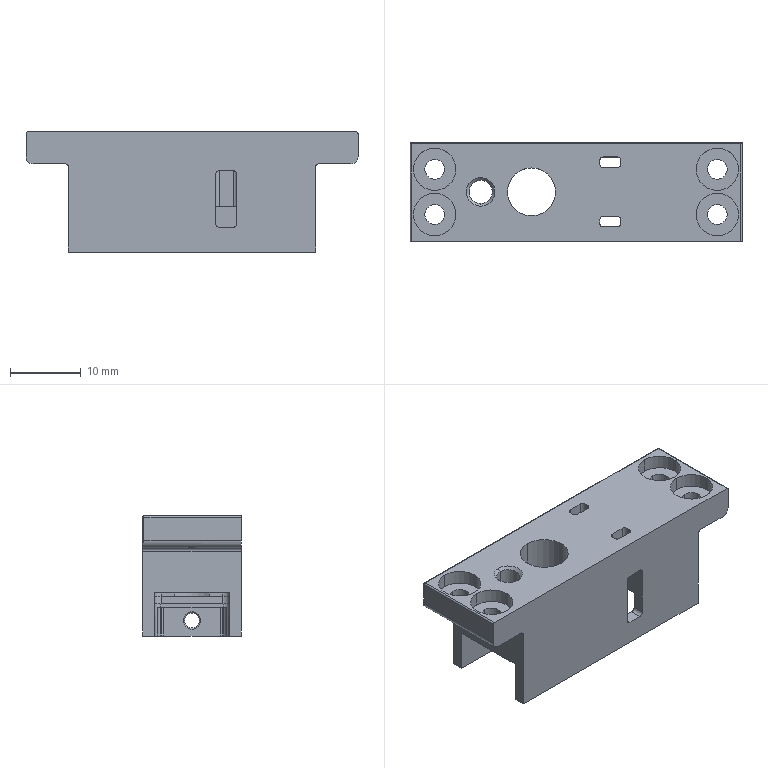NC program | NX | posted with a generic post | part box 47 x 14 x 17 mm
Lines 2950 to 4024 of 12912:
(CAVITY_MILL_COPY_COPY , TOOL : D2)
N5850 T20 M6
N5852 G54
N5854 G17 G0 G90 X8.552 Y-4.05 B0. C0. S9200 M3
N5856 G43 Z30. H20
N5858 Z0.9
N5860 G94 G1 Z-0.1 F1000.
N5862 G3 X9.152 Y-4.25 R1.
N5864 G1 X9.806
N5866 G2 X10.571 Y-3.925 R1.
N5868 X11.027 Y-3.46 R1.14
N5870 G3 X10.654 Y-3.792 R0.5
N5872 G1 X10.528 Y-3.104
N5874 Z0.9
N5876 G0 Z30.
N5878 X8.552 Y-4.05
N5880 Z0.8
N5882 G1 Z-0.2
N5884 G3 X9.152 Y-4.25 R1.
N5886 G1 X9.806
N5888 G2 X10.571 Y-3.925 R1.
N5890 X11.027 Y-3.46 R1.14
N5892 G3 X10.654 Y-3.792 R0.5
N5894 G1 X10.216 Y-3.246
N5896 Z0.8
N5898 G0 Z30.
N5900 X8.552 Y-4.05
N5902 Z0.7
N5904 G1 Z-0.3
N5906 G3 X9.152 Y-4.25 R1.
N5908 G1 X9.806
N5910 G2 X10.571 Y-3.925 R1.
N5912 X11.027 Y-3.46 R1.14
N5914 G3 X10.654 Y-3.792 R0.5
N5916 G1 X10.536 Y-3.102
N5918 Z0.7
N5920 G0 Z30.
N5922 X8.552 Y-4.05
N5924 Z0.6
N5926 G1 Z-0.4
N5928 G3 X9.152 Y-4.25 R1.
N5930 G1 X9.806
N5932 G2 X10.571 Y-3.925 R1.
N5934 X11.027 Y-3.46 R1.14
N5936 G3 X10.654 Y-3.792 R0.5
N5938 G1 X10.216 Y-3.246
N5940 Z0.6
N5942 G0 Z30.
N5944 X8.552 Y-4.05
N5946 Z0.5
N5948 G1 Z-0.5
N5950 G3 X9.152 Y-4.25 R1.
N5952 G1 X9.806
N5954 G2 X10.571 Y-3.925 R1.
N5956 X11.027 Y-3.46 R1.14
N5958 G3 X10.654 Y-3.792 R0.5
N5960 G1 X10.216 Y-3.246
N5962 Z0.5
N5964 G0 Z30.
N5966 X8.552 Y-4.05
N5968 Z0.4
N5970 G1 Z-0.6
N5972 G3 X9.152 Y-4.25 R1.
N5974 G1 X9.806
N5976 G2 X10.571 Y-3.925 R1.
N5978 X11.027 Y-3.46 R1.14
N5980 G3 X10.654 Y-3.792 R0.5
N5982 G1 X10.216 Y-3.246
N5984 Z0.4
N5986 G0 Z30.
N5988 X8.552 Y-4.05
N5990 Z0.3
N5992 G1 Z-0.7
N5994 G3 X9.152 Y-4.25 R1.
N5996 G1 X9.806
N5998 G2 X10.571 Y-3.925 R1.
N6000 X11.027 Y-3.46 R1.14
N6002 G3 X10.654 Y-3.792 R0.5
N6004 G1 X10.216 Y-3.246
N6006 Z0.3
N6008 G0 Z30.
N6010 X8.552 Y-4.05
N6012 Z0.2
N6014 G1 Z-0.8
N6016 G3 X9.152 Y-4.25 R1.
N6018 G1 X9.806
N6020 G2 X10.571 Y-3.925 R1.
N6022 X11.027 Y-3.46 R1.14
N6024 G3 X10.654 Y-3.792 R0.5
N6026 G1 X10.216 Y-3.246
N6028 Z0.2
N6030 G0 Z30.
N6032 X8.552 Y-4.05
N6034 Z0.1
N6036 G1 Z-0.9
N6038 G3 X9.152 Y-4.25 R1.
N6040 G1 X9.806
N6042 G2 X10.571 Y-3.925 R1.
N6044 X11.027 Y-3.46 R1.14
N6046 G3 X10.654 Y-3.792 R0.5
N6048 G1 X10.216 Y-3.246
N6050 Z0.1
N6052 G0 Z30.
N6054 X8.552 Y-4.05
N6056 Z0.
N6058 G1 Z-1.
N6060 G3 X9.152 Y-4.25 R1.
N6062 G1 X9.806
N6064 G2 X10.571 Y-3.925 R1.
N6066 X11.027 Y-3.46 R1.14
N6068 G3 X10.654 Y-3.792 R0.5
N6070 G1 X10.216 Y-3.246
N6072 Z0.
N6074 X8.552 Y-4.05 Z-0.1 F8000.
N6076 Z-1.1 F1000.
N6078 G3 X9.152 Y-4.25 R1.
N6080 G1 X9.806
N6082 G2 X10.571 Y-3.925 R1.
N6084 X11.027 Y-3.46 R1.14
N6086 G3 X10.654 Y-3.792 R0.5
N6088 G1 X10.216 Y-3.246
N6090 Z-0.1
N6092 X8.552 Y-4.05 Z-0.2 F8000.
N6094 Z-1.2 F1000.
N6096 G3 X9.152 Y-4.25 R1.
N6098 G1 X9.806
N6100 G2 X10.571 Y-3.925 R1.
N6102 X11.027 Y-3.46 R1.14
N6104 G3 X10.654 Y-3.792 R0.5
N6106 G1 X10.51 Y-3.107
N6108 Z-0.2
N6110 X8.552 Y-4.05 Z-0.3 F8000.
N6112 Z-1.3 F1000.
N6114 G3 X9.152 Y-4.25 R1.
N6116 G1 X9.806
N6118 G2 X10.571 Y-3.925 R1.
N6120 X11.027 Y-3.46 R1.14
N6122 G3 X10.654 Y-3.792 R0.5
N6124 G1 X10.216 Y-3.246
N6126 Z-0.3
N6128 X8.552 Y-4.05 Z-0.4 F8000.
N6130 Z-1.4 F1000.
N6132 G3 X9.152 Y-4.25 R1.
N6134 G1 X9.806
N6136 G2 X10.571 Y-3.925 R1.
N6138 X11.027 Y-3.46 R1.14
N6140 G3 X10.654 Y-3.792 R0.5
N6142 G1 X10.216 Y-3.246
N6144 Z-0.4
N6146 X8.552 Y-4.05 Z-0.5 F8000.
N6148 Z-1.5 F1000.
N6150 G3 X9.152 Y-4.25 R1.
N6152 G1 X9.806
N6154 G2 X10.571 Y-3.925 R1.
N6156 X11.027 Y-3.46 R1.14
N6158 G3 X10.654 Y-3.792 R0.5
N6160 G1 X10.216 Y-3.246
N6162 Z-0.5
N6164 X8.552 Y-4.05 Z-0.6 F8000.
N6166 Z-1.6 F1000.
N6168 G3 X9.152 Y-4.25 R1.
N6170 G1 X9.806
N6172 G2 X10.571 Y-3.925 R1.
N6174 X11.027 Y-3.46 R1.14
N6176 G3 X10.654 Y-3.792 R0.5
N6178 G1 X10.216 Y-3.246
N6180 Z-0.6
N6182 X8.552 Y-4.05 Z-0.7 F8000.
N6184 Z-1.7 F1000.
N6186 G3 X9.152 Y-4.25 R1.
N6188 G1 X9.806
N6190 G2 X10.571 Y-3.925 R1.
N6192 X11.027 Y-3.46 R1.14
N6194 G3 X10.654 Y-3.792 R0.5
N6196 G1 X10.684 Y-3.093
N6198 Z-0.7
N6200 X8.552 Y-4.05 Z-0.8 F8000.
N6202 Z-1.8 F1000.
N6204 G3 X9.152 Y-4.25 R1.
N6206 G1 X9.806
N6208 G2 X10.571 Y-3.925 R1.
N6210 X11.027 Y-3.46 R1.14
N6212 G3 X10.654 Y-3.792 R0.5
N6214 G1 X10.216 Y-3.246
N6216 Z-0.8
N6218 X8.552 Y-4.05 Z-0.9 F8000.
N6220 Z-1.9 F1000.
N6222 G3 X9.152 Y-4.25 R1.
N6224 G1 X9.806
N6226 G2 X10.571 Y-3.925 R1.
N6228 X11.027 Y-3.46 R1.14
N6230 G3 X10.654 Y-3.792 R0.5
N6232 G1 X10.216 Y-3.246
N6234 Z-0.9
N6236 X8.552 Y-4.05 Z-1. F8000.
N6238 Z-2. F1000.
N6240 G3 X9.152 Y-4.25 R1.
N6242 G1 X9.806
N6244 G2 X10.571 Y-3.925 R1.
N6246 X11.027 Y-3.46 R1.14
N6248 G3 X10.654 Y-3.792 R0.5
N6250 G1 X10.484 Y-3.113
N6252 Z-1.
N6254 X8.552 Y-4.05 Z-1.1 F8000.
N6256 Z-2.1 F1000.
N6258 G3 X9.152 Y-4.25 R1.
N6260 G1 X9.806
N6262 G2 X10.571 Y-3.925 R1.
N6264 X11.027 Y-3.46 R1.14
N6266 G3 X10.654 Y-3.792 R0.5
N6268 G1 X10.216 Y-3.246
N6270 Z-1.1
N6272 X8.552 Y-4.05 Z-1.2 F8000.
N6274 Z-2.2 F1000.
N6276 G3 X9.152 Y-4.25 R1.
N6278 G1 X9.806
N6280 G2 X10.571 Y-3.925 R1.
N6282 X11.027 Y-3.46 R1.14
N6284 G3 X10.654 Y-3.792 R0.5
N6286 G1 X10.216 Y-3.246
N6288 Z-1.2
N6290 X8.552 Y-4.05 Z-1.3 F8000.
N6292 Z-2.3 F1000.
N6294 G3 X9.152 Y-4.25 R1.
N6296 G1 X9.806
N6298 G2 X10.571 Y-3.925 R1.
N6300 X11.027 Y-3.46 R1.14
N6302 G3 X10.654 Y-3.792 R0.5
N6304 G1 X10.216 Y-3.246
N6306 Z-1.3
N6308 X8.552 Y-4.05 Z-1.4 F8000.
N6310 Z-2.4 F1000.
N6312 G3 X9.152 Y-4.25 R1.
N6314 G1 X9.806
N6316 G2 X10.571 Y-3.925 R1.
N6318 X11.027 Y-3.46 R1.14
N6320 G3 X10.654 Y-3.792 R0.5
N6322 G1 X10.216 Y-3.246
N6324 Z-1.4
N6326 X8.552 Y-4.05 Z-1.5 F8000.
N6328 Z-2.5 F1000.
N6330 G3 X9.152 Y-4.25 R1.
N6332 G1 X9.806
N6334 G2 X10.571 Y-3.925 R1.
N6336 X11.027 Y-3.46 R1.14
N6338 G3 X10.654 Y-3.792 R0.5
N6340 G1 X10.216 Y-3.246
N6342 Z-1.5
N6344 X8.552 Y-4.05 Z-1.6 F8000.
N6346 Z-2.6 F1000.
N6348 G3 X9.152 Y-4.25 R1.
N6350 G1 X9.806
N6352 G2 X10.571 Y-3.925 R1.
N6354 X11.027 Y-3.46 R1.14
N6356 G3 X10.654 Y-3.792 R0.5
N6358 G1 X10.216 Y-3.246
N6360 Z-1.6
N6362 X8.552 Y-4.05 Z-1.7 F8000.
N6364 Z-2.7 F1000.
N6366 G3 X9.152 Y-4.25 R1.
N6368 G1 X9.806
N6370 G2 X10.571 Y-3.925 R1.
N6372 X11.027 Y-3.46 R1.14
N6374 G3 X10.654 Y-3.792 R0.5
N6376 G1 X10.506 Y-3.108
N6378 Z-1.7
N6380 X8.552 Y-4.05 Z-1.8 F8000.
N6382 Z-2.8 F1000.
N6384 G3 X9.152 Y-4.25 R1.
N6386 G1 X9.806
N6388 G2 X10.571 Y-3.925 R1.
N6390 X11.027 Y-3.46 R1.14
N6392 G3 X10.654 Y-3.792 R0.5
N6394 G1 X10.591 Y-3.095
N6396 Z-1.8
N6398 X8.552 Y-4.05 Z-1.9 F8000.
N6400 Z-2.9 F1000.
N6402 G3 X9.152 Y-4.25 R1.
N6404 G1 X9.806
N6406 G2 X10.571 Y-3.925 R1.
N6408 X11.027 Y-3.46 R1.14
N6410 G3 X10.654 Y-3.792 R0.5
N6412 G1 X10.555 Y-3.099
N6414 Z-1.9
N6416 X8.552 Y-4.05 Z-2. F8000.
N6418 Z-3. F1000.
N6420 G3 X9.152 Y-4.25 R1.
N6422 G1 X9.806
N6424 G2 X10.571 Y-3.925 R1.
N6426 X11.027 Y-3.46 R1.14
N6428 G3 X10.654 Y-3.792 R0.5
N6430 G1 X10.501 Y-3.109
N6432 Z-2.
N6434 X8.552 Y-4.05 Z-2.1 F8000.
N6436 Z-3.1 F1000.
N6438 G3 X9.152 Y-4.25 R1.
N6440 G1 X9.806
N6442 G2 X10.532 Y-3.925 R1.
N6444 G1 X10.571
N6446 G2 X11.027 Y-3.46 R1.14
N6448 G3 X10.654 Y-3.792 R0.5
N6450 G1 X10.657 Y-3.092
N6452 Z-2.1
N6454 X8.552 Y-4.05 Z-2.2 F8000.
N6456 Z-3.2 F1000.
N6458 G3 X9.152 Y-4.25 R1.
N6460 G1 X9.806
N6462 G2 X10.532 Y-3.925 R1.
N6464 G1 X10.571
N6466 G2 X11.027 Y-3.46 R1.14
N6468 G3 X10.654 Y-3.792 R0.5
N6470 G1 X10.216 Y-3.246
N6472 Z-2.2
N6474 X8.552 Y-4.05 Z-2.3 F8000.
N6476 Z-3.3 F1000.
N6478 G3 X9.152 Y-4.25 R1.
N6480 G1 X9.806
N6482 G2 X10.532 Y-3.925 R1.
N6484 G1 X10.571
N6486 G2 X11.027 Y-3.46 R1.14
N6488 G3 X10.654 Y-3.792 R0.5
N6490 G1 X10.216 Y-3.246
N6492 Z-2.3
N6494 X8.552 Y-4.05 Z-2.4 F8000.
N6496 Z-3.4 F1000.
N6498 G3 X9.152 Y-4.25 R1.
N6500 G1 X9.806
N6502 G2 X10.532 Y-3.925 R1.
N6504 G1 X10.571
N6506 G2 X11.027 Y-3.46 R1.14
N6508 G3 X10.654 Y-3.792 R0.5
N6510 G1 X10.216 Y-3.246
N6512 Z-2.4
N6514 X8.552 Y-4.05 Z-2.5 F8000.
N6516 Z-3.5 F1000.
N6518 G3 X9.152 Y-4.25 R1.
N6520 G1 X9.806
N6522 G2 X10.532 Y-3.925 R1.
N6524 G1 X10.571
N6526 G2 X11.027 Y-3.46 R1.14
N6528 G3 X10.654 Y-3.792 R0.5
N6530 G1 X10.541 Y-3.101
N6532 Z-2.5
N6534 X8.552 Y-4.05 Z-2.6 F8000.
N6536 Z-3.6 F1000.
N6538 G3 X9.152 Y-4.25 R1.
N6540 G1 X9.806
N6542 G2 X10.532 Y-3.925 R1.
N6544 G1 X10.571
N6546 G2 X11.027 Y-3.46 R1.14
N6548 G3 X10.654 Y-3.792 R0.5
N6550 G1 X10.216 Y-3.246
N6552 Z-2.6
N6554 X8.552 Y-4.05 Z-2.7 F8000.
N6556 Z-3.7 F1000.
N6558 G3 X9.152 Y-4.25 R1.
N6560 G1 X9.806
N6562 G2 X10.532 Y-3.925 R1.
N6564 G1 X10.571
N6566 G2 X11.027 Y-3.46 R1.14
N6568 G3 X10.654 Y-3.792 R0.5
N6570 G1 X10.216 Y-3.246
N6572 Z-2.7
N6574 X8.552 Y-4.05 Z-2.8 F8000.
N6576 Z-3.8 F1000.
N6578 G3 X9.152 Y-4.25 R1.
N6580 G1 X9.806
N6582 G2 X10.532 Y-3.925 R1.
N6584 G1 X10.571
N6586 G2 X11.027 Y-3.46 R1.14
N6588 G3 X10.654 Y-3.792 R0.5
N6590 G1 X10.216 Y-3.246
N6592 Z-2.8
N6594 X8.552 Y-4.05 Z-2.9 F8000.
N6596 Z-3.9 F1000.
N6598 G3 X9.152 Y-4.25 R1.
N6600 G1 X9.806
N6602 G2 X10.532 Y-3.925 R1.
N6604 G1 X10.571
N6606 G2 X11.027 Y-3.46 R1.14
N6608 G3 X10.654 Y-3.792 R0.5
N6610 G1 X10.619 Y-3.093
N6612 Z-2.9
N6614 X8.552 Y-4.05 Z-3. F8000.
N6616 Z-4. F1000.
N6618 G3 X9.152 Y-4.25 R1.
N6620 G1 X9.806
N6622 G2 X10.532 Y-3.925 R1.
N6624 G1 X10.571
N6626 G2 X11.027 Y-3.46 R1.14
N6628 G3 X10.654 Y-3.792 R0.5
N6630 G1 X10.216 Y-3.246
N6632 Z-3.
N6634 X8.552 Y-4.05 Z-3.1 F8000.
N6636 Z-4.1 F1000.
N6638 G3 X9.152 Y-4.25 R1.
N6640 G1 X9.806
N6642 G2 X10.532 Y-3.925 R1.
N6644 G1 X10.571
N6646 G2 X11.027 Y-3.46 R1.14
N6648 G3 X10.654 Y-3.792 R0.5
N6650 G1 X10.216 Y-3.246
N6652 Z-3.1
N6654 X7.939 Y-4.137 Z-3.2 F8000.
N6656 Z-4.2 F1000.
N6658 G3 X8.401 Y-4.25 R1.
N6660 G1 X9.7
N6662 Y-2.951
N6664 G3 X9.5 Y-2.351 R1.
N6666 G1 Z-3.2
N6668 X7.939 Y-4.137 Z-3.3 F8000.
N6670 Z-4.3 F1000.
N6672 G3 X8.401 Y-4.25 R1.
N6674 G1 X9.7
N6676 Y-2.951
N6678 G3 X9.5 Y-2.351 R1.
N6680 G1 Z-3.3
N6682 X7.939 Y-4.137 Z-3.4 F8000.
N6684 Z-4.4 F1000.
N6686 G3 X8.401 Y-4.25 R1.
N6688 G1 X9.7
N6690 Y-2.951
N6692 G3 X9.5 Y-2.351 R1.
N6694 G1 Z-3.4
N6696 X7.939 Y-4.137 Z-3.5 F8000.
N6698 Z-4.5 F1000.
N6700 G3 X8.401 Y-4.25 R1.
N6702 G1 X9.7
N6704 Y-2.951
N6706 G3 X9.5 Y-2.351 R1.
N6708 G1 Z-3.5
N6710 X7.939 Y-4.137 Z-3.6 F8000.
N6712 Z-4.6 F1000.
N6714 G3 X8.401 Y-4.25 R1.
N6716 G1 X9.7
N6718 Y-2.951
N6720 G3 X9.5 Y-2.351 R1.
N6722 G1 Z-3.6
N6724 X7.939 Y-4.137 Z-3.7 F8000.
N6726 Z-4.7 F1000.
N6728 G3 X8.401 Y-4.25 R1.
N6730 G1 X9.7
N6732 Y-2.951
N6734 G3 X9.5 Y-2.351 R1.
N6736 G1 Z-3.7
N6738 X7.939 Y-4.137 Z-3.8 F8000.
N6740 Z-4.8 F1000.
N6742 G3 X8.401 Y-4.25 R1.
N6744 G1 X9.7
N6746 Y-2.951
N6748 G3 X9.5 Y-2.351 R1.
N6750 G1 Z-3.8
N6752 X7.939 Y-4.137 Z-3.9 F8000.
N6754 Z-4.9 F1000.
N6756 G3 X8.401 Y-4.25 R1.
N6758 G1 X9.7
N6760 Y-2.951
N6762 G3 X9.5 Y-2.351 R1.
N6764 G1 Z-3.9
N6766 X7.939 Y-4.137 Z-4. F8000.
N6768 Z-5. F1000.
N6770 G3 X8.401 Y-4.25 R1.
N6772 G1 X9.7
N6774 Y-2.951
N6776 G3 X9.5 Y-2.351 R1.
N6778 G1 Z-4.
N6780 X7.939 Y-4.137 Z-4.1 F8000.
N6782 Z-5.1 F1000.
N6784 G3 X8.401 Y-4.25 R1.
N6786 G1 X9.7
N6788 Y-2.951
N6790 G3 X9.5 Y-2.351 R1.
N6792 G1 Z-4.1
N6794 X7.939 Y-4.137 Z-4.2 F8000.
N6796 Z-5.2 F1000.
N6798 G3 X8.401 Y-4.25 R1.
N6800 G1 X9.7
N6802 Y-2.951
N6804 G3 X9.5 Y-2.351 R1.
N6806 G1 Z-4.2
N6808 X7.939 Y-4.137 Z-4.3 F8000.
N6810 Z-5.3 F1000.
N6812 G3 X8.401 Y-4.25 R1.
N6814 G1 X9.7
N6816 Y-2.951
N6818 G3 X9.5 Y-2.351 R1.
N6820 G1 Z-4.3
N6822 X7.939 Y-4.137 Z-4.4 F8000.
N6824 Z-5.4 F1000.
N6826 G3 X8.401 Y-4.25 R1.
N6828 G1 X9.7
N6830 Y-2.951
N6832 G3 X9.5 Y-2.351 R1.
N6834 G1 Z-4.4
N6836 X7.939 Y-4.137 Z-4.5 F8000.
N6838 Z-5.5 F1000.
N6840 G3 X8.401 Y-4.25 R1.
N6842 G1 X9.7
N6844 Y-2.951
N6846 G3 X9.5 Y-2.351 R1.
N6848 G1 Z-4.5
N6850 X7.939 Y-4.137 Z-4.6 F8000.
N6852 Z-5.6 F1000.
N6854 G3 X8.401 Y-4.25 R1.
N6856 G1 X9.7
N6858 Y-2.951
N6860 G3 X9.5 Y-2.351 R1.
N6862 G1 Z-4.6
N6864 X7.939 Y-4.137 Z-4.7 F8000.
N6866 Z-5.7 F1000.
N6868 G3 X8.401 Y-4.25 R1.
N6870 G1 X9.7
N6872 Y-2.951
N6874 G3 X9.5 Y-2.351 R1.
N6876 G1 Z-4.7
N6878 X7.939 Y-4.137 Z-4.8 F8000.
N6880 Z-5.8 F1000.
N6882 G3 X8.401 Y-4.25 R1.
N6884 G1 X9.7
N6886 Y-2.951
N6888 G3 X9.5 Y-2.351 R1.
N6890 G1 Z-4.8
N6892 X7.939 Y-4.137 Z-4.9 F8000.
N6894 Z-5.9 F1000.
N6896 G3 X8.401 Y-4.25 R1.
N6898 G1 X9.7
N6900 Y-2.951
N6902 G3 X9.5 Y-2.351 R1.
N6904 G1 Z-4.9
N6906 X7.939 Y-4.137 Z-5. F8000.
N6908 Z-6. F1000.
N6910 G3 X8.401 Y-4.25 R1.
N6912 G1 X9.7
N6914 Y-2.951
N6916 G3 X9.5 Y-2.351 R1.
N6918 G1 Z-5.
N6920 X7.939 Y-4.137 Z-5.1 F8000.
N6922 Z-6.1 F1000.
N6924 G3 X8.401 Y-4.25 R1.
N6926 G1 X9.7
N6928 Y-2.951
N6930 G3 X9.5 Y-2.351 R1.
N6932 G1 Z-5.1
N6934 X7.939 Y-4.137 Z-5.2 F8000.
N6936 Z-6.2 F1000.
N6938 G3 X8.401 Y-4.25 R1.
N6940 G1 X9.7
N6942 Y-2.951
N6944 G3 X9.5 Y-2.351 R1.
N6946 G1 Z-5.2
N6948 X7.939 Y-4.137 Z-5.3 F8000.
N6950 Z-6.3 F1000.
N6952 G3 X8.401 Y-4.25 R1.
N6954 G1 X9.7
N6956 Y-2.951
N6958 G3 X9.5 Y-2.351 R1.
N6960 G1 Z-5.3
N6962 X7.939 Y-4.137 Z-5.4 F8000.
N6964 Z-6.4 F1000.
N6966 G3 X8.401 Y-4.25 R1.
N6968 G1 X9.7
N6970 Y-2.951
N6972 G3 X9.5 Y-2.351 R1.
N6974 G1 Z-5.4
N6976 X7.939 Y-4.137 Z-5.5 F8000.
N6978 Z-6.5 F1000.
N6980 G3 X8.401 Y-4.25 R1.
N6982 G1 X9.7
N6984 Y-2.951
N6986 G3 X9.5 Y-2.351 R1.
N6988 G1 Z-5.5
N6990 G0 Z30.
N6992 X9.984 Y-3.385
N6994 Z0.9
N6996 G1 Z-0.1
N6998 X10.042 Y-3.421
N7000 G3 X11.041 Y-3.453 R1.
N7002 G2 X12.2 Y-3.502 R1.14
N7004 G1 Y-2.053
N7006 G3 X12. Y-1.453 R1.
N7008 G1 Z0.9
N7010 G0 Z30.
N7012 X9.984 Y-3.385
N7014 Z0.8
N7016 G1 Z-0.2
N7018 X10.042 Y-3.421
N7020 G3 X11.041 Y-3.453 R1.
N7022 G2 X12.2 Y-3.502 R1.14
N7024 G1 Y-2.053
N7026 G3 X12. Y-1.453 R1.
N7028 G1 Z0.8
N7030 G0 Z30.
N7032 X9.984 Y-3.385
N7034 Z0.7
N7036 G1 Z-0.3
N7038 X10.042 Y-3.421
N7040 G3 X11.041 Y-3.453 R1.
N7042 G2 X12.2 Y-3.502 R1.14
N7044 G1 Y-2.053
N7046 G3 X12. Y-1.453 R1.
N7048 G1 Z0.7
N7050 G0 Z30.
N7052 X9.984 Y-3.385
N7054 Z0.6
N7056 G1 Z-0.4
N7058 X10.042 Y-3.421
N7060 G3 X11.041 Y-3.453 R1.
N7062 G2 X12.2 Y-3.502 R1.14
N7064 G1 Y-2.053
N7066 G3 X12. Y-1.453 R1.
N7068 G1 Z0.6
N7070 G0 Z30.
N7072 X9.984 Y-3.385
N7074 Z0.5
N7076 G1 Z-0.5
N7078 X10.042 Y-3.421
N7080 G3 X11.041 Y-3.453 R1.
N7082 G2 X12.2 Y-3.502 R1.14
N7084 G1 Y-2.053
N7086 G3 X12. Y-1.453 R1.
N7088 G1 Z0.5
N7090 G0 Z30.
N7092 X9.984 Y-3.385
N7094 Z0.4
N7096 G1 Z-0.6
N7098 X10.042 Y-3.421
N7100 G3 X11.041 Y-3.453 R1.
N7102 G2 X12.2 Y-3.502 R1.14
N7104 G1 Y-2.053
N7106 G3 X12. Y-1.453 R1.
N7108 G1 Z0.4
N7110 G0 Z30.
N7112 X9.984 Y-3.385
N7114 Z0.3
N7116 G1 Z-0.7
N7118 X10.042 Y-3.421
N7120 G3 X11.041 Y-3.453 R1.
N7122 G2 X12.2 Y-3.502 R1.14
N7124 G1 Y-2.053
N7126 G3 X12. Y-1.453 R1.
N7128 G1 Z0.3
N7130 G0 Z30.
N7132 X9.984 Y-3.385
N7134 Z0.2
N7136 G1 Z-0.8
N7138 X10.042 Y-3.421
N7140 G3 X11.041 Y-3.453 R1.
N7142 G2 X12.2 Y-3.502 R1.14
N7144 G1 Y-2.053
N7146 G3 X12. Y-1.453 R1.
N7148 G1 Z0.2
N7150 G0 Z30.
N7152 X9.984 Y-3.385
N7154 Z0.1
N7156 G1 Z-0.9
N7158 X10.042 Y-3.421
N7160 G3 X11.041 Y-3.453 R1.
N7162 G2 X12.2 Y-3.502 R1.14
N7164 G1 Y-2.053
N7166 G3 X12. Y-1.453 R1.
N7168 G1 Z0.1
N7170 G0 Z30.
N7172 X9.984 Y-3.385
N7174 Z0.
N7176 G1 Z-1.
N7178 X10.042 Y-3.421
N7180 G3 X11.041 Y-3.453 R1.
N7182 G2 X12.2 Y-3.502 R1.14
N7184 G1 Y-2.053
N7186 G3 X12. Y-1.453 R1.
N7188 G1 Z0.
N7190 X9.984 Y-3.385 Z-0.1 F8000.
N7192 Z-1.1 F1000.
N7194 X10.042 Y-3.421
N7196 G3 X11.041 Y-3.453 R1.
N7198 G2 X12.2 Y-3.502 R1.14
N7200 G1 Y-2.053
N7202 G3 X12. Y-1.453 R1.
N7204 G1 Z-0.1
N7206 X9.984 Y-3.385 Z-0.2 F8000.
N7208 Z-1.2 F1000.
N7210 X10.042 Y-3.421
N7212 G3 X11.041 Y-3.453 R1.
N7214 G2 X12.2 Y-3.502 R1.14
N7216 G1 Y-2.053
N7218 G3 X12. Y-1.453 R1.
N7220 G1 Z-0.2
N7222 X9.984 Y-3.385 Z-0.3 F8000.
N7224 Z-1.3 F1000.
N7226 X10.042 Y-3.421
N7228 G3 X11.041 Y-3.453 R1.
N7230 G2 X12.2 Y-3.502 R1.14
N7232 G1 Y-2.053
N7234 G3 X12. Y-1.453 R1.
N7236 G1 Z-0.3
N7238 X9.984 Y-3.385 Z-0.4 F8000.
N7240 Z-1.4 F1000.
N7242 X10.042 Y-3.421
N7244 G3 X11.041 Y-3.453 R1.
N7246 G2 X12.2 Y-3.502 R1.14
N7248 G1 Y-2.053
N7250 G3 X12. Y-1.453 R1.
N7252 G1 Z-0.4
N7254 X9.984 Y-3.385 Z-0.5 F8000.
N7256 Z-1.5 F1000.
N7258 X10.042 Y-3.421
N7260 G3 X11.041 Y-3.453 R1.
N7262 G2 X12.2 Y-3.502 R1.14
N7264 G1 Y-2.053
N7266 G3 X12. Y-1.453 R1.
N7268 G1 Z-0.5
N7270 X9.984 Y-3.385 Z-0.6 F8000.
N7272 Z-1.6 F1000.
N7274 X10.042 Y-3.421
N7276 G3 X11.041 Y-3.453 R1.
N7278 G2 X12.2 Y-3.502 R1.14
N7280 G1 Y-2.053
N7282 G3 X12. Y-1.453 R1.
N7284 G1 Z-0.6
N7286 X9.984 Y-3.385 Z-0.7 F8000.
N7288 Z-1.7 F1000.
N7290 X10.042 Y-3.421
N7292 G3 X11.041 Y-3.453 R1.
N7294 G2 X12.2 Y-3.502 R1.14
N7296 G1 Y-2.053
N7298 G3 X12. Y-1.453 R1.
N7300 G1 Z-0.7
N7302 X9.984 Y-3.385 Z-0.8 F8000.
N7304 Z-1.8 F1000.
N7306 X10.042 Y-3.421
N7308 G3 X11.041 Y-3.453 R1.
N7310 G2 X12.2 Y-3.502 R1.14
N7312 G1 Y-2.053
N7314 G3 X12. Y-1.453 R1.
N7316 G1 Z-0.8
N7318 X9.984 Y-3.385 Z-0.9 F8000.
N7320 Z-1.9 F1000.
N7322 X10.042 Y-3.421
N7324 G3 X11.041 Y-3.453 R1.
N7326 G2 X12.2 Y-3.502 R1.14
N7328 G1 Y-2.053
N7330 G3 X12. Y-1.453 R1.
N7332 G1 Z-0.9
N7334 X9.984 Y-3.385 Z-1. F8000.
N7336 Z-2. F1000.
N7338 X10.042 Y-3.421
N7340 G3 X11.041 Y-3.453 R1.
N7342 G2 X12.2 Y-3.502 R1.14
N7344 G1 Y-2.053
N7346 G3 X12. Y-1.453 R1.
N7348 G1 Z-1.
N7350 X9.984 Y-3.385 Z-1.1 F8000.
N7352 Z-2.1 F1000.
N7354 X10.042 Y-3.421
N7356 G3 X11.041 Y-3.453 R1.
N7358 G2 X12.2 Y-3.502 R1.14
N7360 G1 Y-2.053
N7362 G3 X12. Y-1.453 R1.
N7364 G1 Z-1.1
N7366 X9.984 Y-3.385 Z-1.2 F8000.
N7368 Z-2.2 F1000.
N7370 X10.042 Y-3.421
N7372 G3 X11.041 Y-3.453 R1.
N7374 G2 X12.2 Y-3.502 R1.14
N7376 G1 Y-2.053
N7378 G3 X12. Y-1.453 R1.
N7380 G1 Z-1.2
N7382 X9.984 Y-3.385 Z-1.3 F8000.
N7384 Z-2.3 F1000.
N7386 X10.042 Y-3.421
N7388 G3 X11.041 Y-3.453 R1.
N7390 G2 X12.2 Y-3.502 R1.14
N7392 G1 Y-2.053
N7394 G3 X12. Y-1.453 R1.
N7396 G1 Z-1.3
N7398 X9.984 Y-3.385 Z-1.4 F8000.
N7400 Z-2.4 F1000.
N7402 X10.042 Y-3.421
N7404 G3 X11.041 Y-3.453 R1.
N7406 G2 X12.2 Y-3.502 R1.14
N7408 G1 Y-2.053
N7410 G3 X12. Y-1.453 R1.
N7412 G1 Z-1.4
N7414 X9.984 Y-3.385 Z-1.5 F8000.
N7416 Z-2.5 F1000.
N7418 X10.042 Y-3.421
N7420 G3 X11.041 Y-3.453 R1.
N7422 G2 X12.2 Y-3.502 R1.14
N7424 G1 Y-2.053
N7426 G3 X12. Y-1.453 R1.
N7428 G1 Z-1.5
N7430 X9.984 Y-3.385 Z-1.6 F8000.
N7432 Z-2.6 F1000.
N7434 X10.042 Y-3.421
N7436 G3 X11.041 Y-3.453 R1.
N7438 G2 X12.2 Y-3.502 R1.14
N7440 G1 Y-2.053
N7442 G3 X12. Y-1.453 R1.
N7444 G1 Z-1.6
N7446 X9.984 Y-3.385 Z-1.7 F8000.
N7448 Z-2.7 F1000.
N7450 X10.042 Y-3.421
N7452 G3 X11.041 Y-3.453 R1.
N7454 G2 X12.2 Y-3.502 R1.14
N7456 G1 Y-2.053
N7458 G3 X12. Y-1.453 R1.
N7460 G1 Z-1.7
N7462 X9.984 Y-3.385 Z-1.8 F8000.
N7464 Z-2.8 F1000.
N7466 X10.042 Y-3.421
N7468 G3 X11.041 Y-3.453 R1.
N7470 G2 X12.2 Y-3.502 R1.14
N7472 G1 Y-2.053
N7474 G3 X12. Y-1.453 R1.
N7476 G1 Z-1.8
N7478 X9.984 Y-3.385 Z-1.9 F8000.
N7480 Z-2.9 F1000.
N7482 X10.042 Y-3.421
N7484 G3 X11.041 Y-3.453 R1.
N7486 G2 X12.2 Y-3.502 R1.14
N7488 G1 Y-2.053
N7490 G3 X12. Y-1.453 R1.
N7492 G1 Z-1.9
N7494 X9.984 Y-3.385 Z-2. F8000.
N7496 Z-3. F1000.
N7498 X10.042 Y-3.421
N7500 G3 X11.041 Y-3.453 R1.
N7502 G2 X12.2 Y-3.502 R1.14
N7504 G1 Y-2.053
N7506 G3 X12. Y-1.453 R1.
N7508 G1 Z-2.
N7510 X9.984 Y-3.385 Z-2.1 F8000.
N7512 Z-3.1 F1000.
N7514 X10.042 Y-3.421
N7516 G3 X11.041 Y-3.453 R1.
N7518 G2 X12.2 Y-3.502 R1.14
N7520 G1 Y-2.053
N7522 G3 X12. Y-1.453 R1.
N7524 G1 Z-2.1
N7526 X9.984 Y-3.385 Z-2.2 F8000.
N7528 Z-3.2 F1000.
N7530 X10.042 Y-3.421
N7532 G3 X11.041 Y-3.453 R1.
N7534 G2 X12.2 Y-3.502 R1.14
N7536 G1 Y-2.053
N7538 G3 X12. Y-1.453 R1.
N7540 G1 Z-2.2
N7542 X9.984 Y-3.385 Z-2.3 F8000.
N7544 Z-3.3 F1000.
N7546 X10.042 Y-3.421
N7548 G3 X11.041 Y-3.453 R1.
N7550 G2 X12.2 Y-3.502 R1.14
N7552 G1 Y-2.053
N7554 G3 X12. Y-1.453 R1.
N7556 G1 Z-2.3
N7558 X9.984 Y-3.385 Z-2.4 F8000.
N7560 Z-3.4 F1000.
N7562 X10.042 Y-3.421
N7564 G3 X11.041 Y-3.453 R1.
N7566 G2 X12.2 Y-3.502 R1.14
N7568 G1 Y-2.053
N7570 G3 X12. Y-1.453 R1.
N7572 G1 Z-2.4
N7574 X9.984 Y-3.385 Z-2.5 F8000.
N7576 Z-3.5 F1000.
N7578 X10.042 Y-3.421
N7580 G3 X11.041 Y-3.453 R1.
N7582 G2 X12.2 Y-3.502 R1.14
N7584 G1 Y-2.053
N7586 G3 X12. Y-1.453 R1.
N7588 G1 Z-2.5
N7590 X9.984 Y-3.385 Z-2.6 F8000.
N7592 Z-3.6 F1000.
N7594 X10.042 Y-3.421
N7596 G3 X11.041 Y-3.453 R1.
N7598 G2 X12.2 Y-3.502 R1.14
N7600 G1 Y-2.053
N7602 G3 X12. Y-1.453 R1.
N7604 G1 Z-2.6
N7606 X9.984 Y-3.385 Z-2.7 F8000.
N7608 Z-3.7 F1000.
N7610 X10.042 Y-3.421
N7612 G3 X11.041 Y-3.453 R1.
N7614 G2 X12.2 Y-3.502 R1.14
N7616 G1 Y-2.053
N7618 G3 X12. Y-1.453 R1.
N7620 G1 Z-2.7
N7622 X9.984 Y-3.385 Z-2.8 F8000.
N7624 Z-3.8 F1000.
N7626 X10.042 Y-3.421
N7628 G3 X11.041 Y-3.453 R1.
N7630 G2 X12.2 Y-3.502 R1.14
N7632 G1 Y-2.053
N7634 G3 X12. Y-1.453 R1.
N7636 G1 Z-2.8
N7638 X9.984 Y-3.385 Z-2.9 F8000.
N7640 Z-3.9 F1000.
N7642 X10.042 Y-3.421
N7644 G3 X11.041 Y-3.453 R1.
N7646 G2 X12.2 Y-3.502 R1.14
N7648 G1 Y-2.053
N7650 G3 X12. Y-1.453 R1.
N7652 G1 Z-2.9
N7654 X9.984 Y-3.385 Z-3. F8000.
N7656 Z-4. F1000.
N7658 X10.042 Y-3.421
N7660 G3 X11.041 Y-3.453 R1.
N7662 G2 X12.2 Y-3.502 R1.14
N7664 G1 Y-2.053
N7666 G3 X12. Y-1.453 R1.
N7668 G1 Z-3.
N7670 X9.984 Y-3.385 Z-3.1 F8000.
N7672 Z-4.1 F1000.
N7674 X10.042 Y-3.421
N7676 G3 X11.041 Y-3.453 R1.
N7678 G2 X12.2 Y-3.502 R1.14
N7680 G1 Y-2.053
N7682 G3 X12. Y-1.453 R1.
N7684 G1 Z-3.1
N7686 G0 Z30.
N7688 Y1.453
N7690 Z0.9
N7692 G1 Z-0.1
N7694 G3 X12.2 Y2.053 R1.
N7696 G1 Y3.502
N7698 X12.191 Y3.518
N7700 G2 X11.585 Y3.318 R1.14
N7702 X11.041 Y3.453 R1.14
N7704 G3 X11.523 Y3.319 R0.5
N7706 G1 X11.103 Y2.759
N7708 Z0.9
N7710 G0 Z30.
N7712 X12. Y1.453
N7714 Z0.8
N7716 G1 Z-0.2
N7718 G3 X12.2 Y2.053 R1.
N7720 G1 Y3.502
N7722 X12.191 Y3.518
N7724 G2 X11.585 Y3.318 R1.14
N7726 X11.041 Y3.453 R1.14
N7728 G3 X11.523 Y3.319 R0.5
N7730 G1 X10.852 Y3.121
N7732 Z0.8
N7734 G0 Z30.
N7736 X12. Y1.453
N7738 Z0.7
N7740 G1 Z-0.3
N7742 G3 X12.2 Y2.053 R1.
N7744 G1 Y3.502
N7746 X12.191 Y3.518
N7748 G2 X11.585 Y3.318 R1.14
N7750 X11.041 Y3.453 R1.14
N7752 G3 X11.523 Y3.319 R0.5
N7754 G1 X11.301 Y2.655
N7756 Z0.7
N7758 G0 Z30.
N7760 X12. Y1.453
N7762 Z0.6
N7764 G1 Z-0.4
N7766 G3 X12.2 Y2.053 R1.
N7768 G1 Y3.502
N7770 X12.191 Y3.518
N7772 G2 X11.585 Y3.318 R1.14
N7774 X11.041 Y3.453 R1.14
N7776 G3 X11.523 Y3.319 R0.5
N7778 G1 X11.301 Y2.655
N7780 Z0.6
N7782 G0 Z30.
N7784 X12. Y1.453
N7786 Z0.5
N7788 G1 Z-0.5
N7790 G3 X12.2 Y2.053 R1.
N7792 G1 Y3.502
N7794 X12.191 Y3.518
N7796 G2 X11.585 Y3.318 R1.14
N7798 X11.041 Y3.453 R1.14
N7800 G3 X11.523 Y3.319 R0.5
N7802 G1 X11.301 Y2.655
N7804 Z0.5
N7806 G0 Z30.
N7808 X12. Y1.453
N7810 Z0.4
N7812 G1 Z-0.6
N7814 G3 X12.2 Y2.053 R1.
N7816 G1 Y3.502
N7818 X12.191 Y3.518
N7820 G2 X11.585 Y3.318 R1.14
N7822 X11.041 Y3.453 R1.14
N7824 G3 X11.523 Y3.319 R0.5
N7826 G1 X10.852 Y3.121
N7828 Z0.4
N7830 G0 Z30.
N7832 X12. Y1.453
N7834 Z0.3
N7836 G1 Z-0.7
N7838 G3 X12.2 Y2.053 R1.
N7840 G1 Y3.502
N7842 X12.191 Y3.518
N7844 G2 X11.585 Y3.318 R1.14
N7846 X11.041 Y3.453 R1.14
N7848 G3 X11.523 Y3.319 R0.5
N7850 G1 X11.301 Y2.655
N7852 Z0.3
N7854 G0 Z30.
N7856 X12. Y1.453
N7858 Z0.2
N7860 G1 Z-0.8
N7862 G3 X12.2 Y2.053 R1.
N7864 G1 Y3.502
N7866 X12.191 Y3.518
N7868 G2 X11.585 Y3.318 R1.14
N7870 X11.041 Y3.453 R1.14
N7872 G3 X11.523 Y3.319 R0.5
N7874 G1 X11.029 Y2.823
N7876 Z0.2
N7878 G0 Z30.
N7880 X12. Y1.453
N7882 Z0.1
N7884 G1 Z-0.9
N7886 G3 X12.2 Y2.053 R1.
N7888 G1 Y3.502
N7890 X12.191 Y3.518
N7892 G2 X11.585 Y3.318 R1.14
N7894 X11.041 Y3.453 R1.14
N7896 G3 X11.523 Y3.319 R0.5
N7898 G1 X10.852 Y3.121
N7900 Z0.1
N7902 G0 Z30.
N7904 X12. Y1.453
N7906 Z0.
N7908 G1 Z-1.
N7910 G3 X12.2 Y2.053 R1.
N7912 G1 Y3.502
N7914 X12.191 Y3.518
N7916 G2 X11.585 Y3.318 R1.14
N7918 X11.041 Y3.453 R1.14
N7920 G3 X11.523 Y3.319 R0.5
N7922 G1 X11.037 Y2.815
N7924 Z0.
N7926 X12. Y1.453 Z-0.1 F8000.
N7928 Z-1.1 F1000.
N7930 G3 X12.2 Y2.053 R1.
N7932 G1 Y3.502
N7934 X12.191 Y3.518
N7936 G2 X11.585 Y3.318 R1.14
N7938 X11.041 Y3.453 R1.14
N7940 G3 X11.523 Y3.319 R0.5
N7942 G1 X10.905 Y2.99
N7944 Z-0.1
N7946 X12. Y1.453 Z-0.2 F8000.
N7948 Z-1.2 F1000.
N7950 G3 X12.2 Y2.053 R1.
N7952 G1 Y3.502
N7954 X12.191 Y3.518
N7956 G2 X11.585 Y3.318 R1.14
N7958 X11.041 Y3.453 R1.14
N7960 G3 X11.523 Y3.319 R0.5
N7962 G1 X11.002 Y2.852
N7964 Z-0.2
N7966 X12. Y1.453 Z-0.3 F8000.
N7968 Z-1.3 F1000.
N7970 G3 X12.2 Y2.053 R1.
N7972 G1 Y3.502
N7974 X12.191 Y3.518
N7976 G2 X11.585 Y3.318 R1.14
N7978 X11.041 Y3.453 R1.14
N7980 G3 X11.523 Y3.319 R0.5
N7982 G1 X11.301 Y2.655
N7984 Z-0.3
N7986 X12. Y1.453 Z-0.4 F8000.
N7988 Z-1.4 F1000.
N7990 G3 X12.2 Y2.053 R1.
N7992 G1 Y3.502